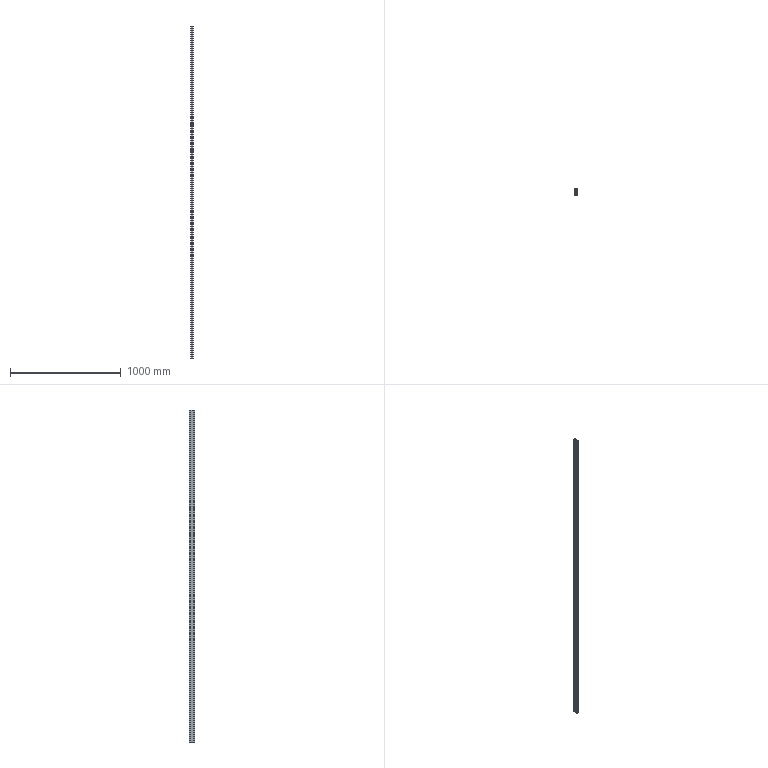Part | STEP file | HFS5-2550-3000 | 1 solid | 230 faces | box 25 x 50.001 x 3000 mm | volume 1510106 mm3 | plane 136 | cylinder 94 | commonest cylinder face diameters 0.6 x30 2.6 x24 2 x13 1.4 x10 6.8 x10 3 x4